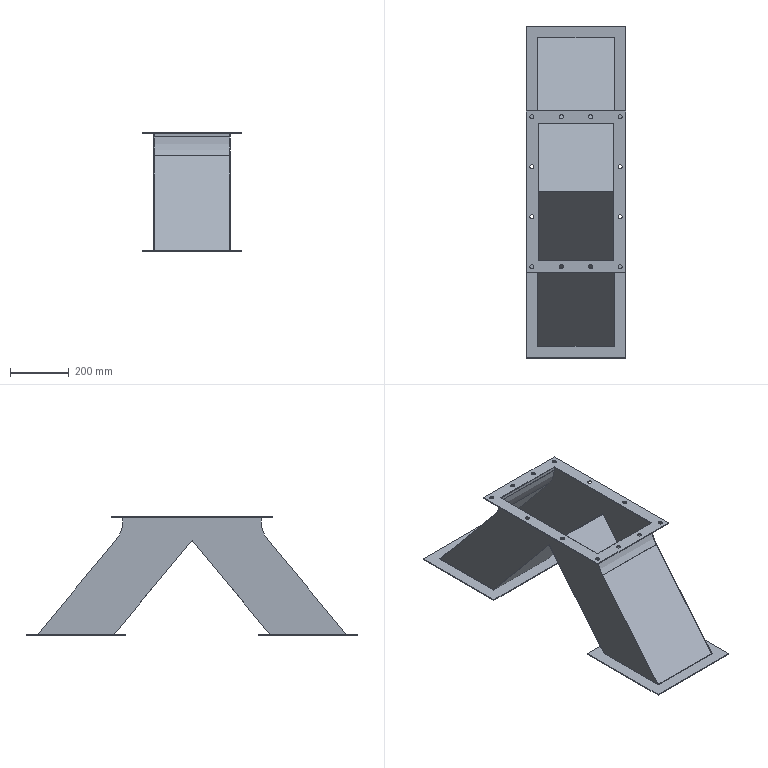Part | STEP file | Produce dryer line heating fan-OVEN-422 | 3 solids | 72 faces | box 340 x 1130 x 403 mm | volume 1800056 mm3 | plane 44 | cylinder 28 | commonest cylinder face diameters 14 x24 200 x2 203 x2